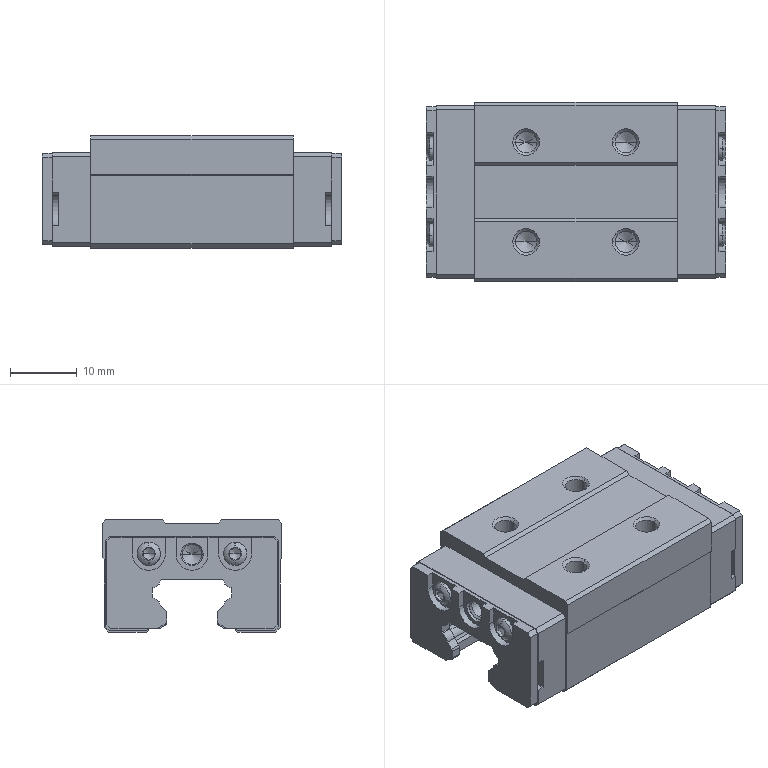Part | NX | 1 solid | 368 faces | box 45 x 27 x 16.9 mm | volume 14821 mm3 | plane 218 | cylinder 102 | cone 32 | torus 16 | commonest cylinder face diameters 1 x20 2.6 x16 2 x8 2.24 x8 2.48 x8 3.5 x8